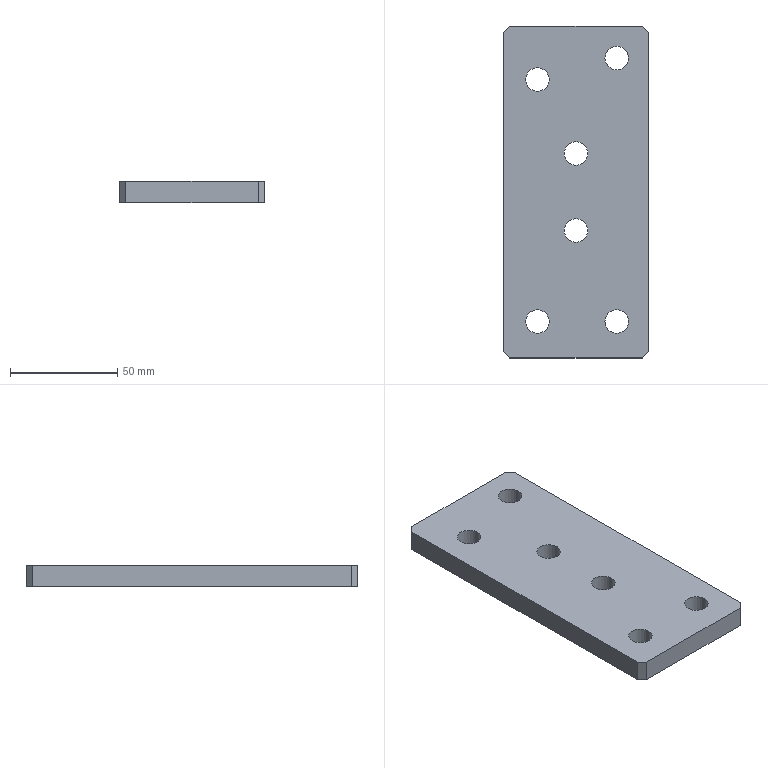Part | STEP file | 1_id186_x_t | 1 solid | 16 faces | box 68 x 155 x 10 mm | volume 99518 mm3 | plane 10 | cylinder 6 | commonest cylinder face diameters 11 x6
STEP:
#1=CARTESIAN_POINT('',(0.,0.,0.));
#2=DIRECTION('',(0.,0.,1.));
#3=DIRECTION('',(1.,0.,0.));
#4=AXIS2_PLACEMENT_3D('',#1,#2,#3);
#5=CARTESIAN_POINT('',(51.775,230.,100.11));
#6=VERTEX_POINT('',#5);
#7=CARTESIAN_POINT('',(46.275,230.,100.11));
#8=DIRECTION('',(0.,0.,-1.));
#9=DIRECTION('',(1.,0.,0.));
#10=AXIS2_PLACEMENT_3D('',#7,#8,#9);
#11=CIRCLE('',#10,5.5);
#12=CARTESIAN_POINT('',(46.275,230.,-100.11));
#13=DIRECTION('',(0.,0.,1.));
#14=DIRECTION('',(1.,0.,0.));
#15=AXIS2_PLACEMENT_3D('',#12,#13,#14);
#16=CYLINDRICAL_SURFACE('',#15,5.5);
#17=CARTESIAN_POINT('',(6.283,200.22));
#18=DIRECTION('',(-1.,0.));
#19=VECTOR('',#18,1.);
#20=LINE('',#17,#19);
#21=(GEOMETRIC_REPRESENTATION_CONTEXT(2)PARAMETRIC_REPRESENTATION_CONTEXT()REPRESENTATION_CONTEXT('',''));
#22=DEFINITIONAL_REPRESENTATION('',(#20),#21);
#23=PCURVE('',#16,#22);
#24=CARTESIAN_POINT('',(96.738,255.,100.11));
#25=DIRECTION('',(0.,0.,1.));
#26=DIRECTION('',(1.,0.,0.));
#27=AXIS2_PLACEMENT_3D('',#24,#25,#26);
#28=PLANE('',#27);
#29=CARTESIAN_POINT('',(-44.962,-25.));
#30=CARTESIAN_POINT('',(-44.962,-34.526));
#31=CARTESIAN_POINT('',(-53.212,-29.763));
#32=CARTESIAN_POINT('',(-61.462,-25.));
#33=CARTESIAN_POINT('',(-53.212,-20.237));
#34=CARTESIAN_POINT('',(-44.962,-15.474));
#35=CARTESIAN_POINT('',(-44.962,-25.));
#36=(BOUNDED_CURVE()B_SPLINE_CURVE(2,(#29,#30,#31,#32,#33,#34,#35),.UNSPECIFIED.,.T.,.F.)B_SPLINE_CURVE_WITH_KNOTS((1,2,2,2,2,1),(-2.094,0.,2.094,4.189,6.283,8.378),.UNSPECIFIED.)CURVE()GEOMETRIC_REPRESENTATION_ITEM()RATIONAL_B_SPLINE_CURVE((1.,0.5,1.,0.5,1.,0.5,1.))REPRESENTATION_ITEM(''));
#37=(GEOMETRIC_REPRESENTATION_CONTEXT(2)PARAMETRIC_REPRESENTATION_CONTEXT()REPRESENTATION_CONTEXT('',''));
#38=DEFINITIONAL_REPRESENTATION('',(#36),#37);
#39=PCURVE('',#28,#38);
#40=SURFACE_CURVE('',#11,(#23,#39),.PCURVE_S1.);
#41=EDGE_CURVE('',#6,#6,#40,.T.);
#42=ORIENTED_EDGE('',*,*,#41,.T.);
#43=CARTESIAN_POINT('',(51.775,230.,90.11));
#44=VERTEX_POINT('',#43);
#45=CARTESIAN_POINT('',(51.775,230.,90.11));
#46=CARTESIAN_POINT('',(51.775,230.,100.11));
#47=B_SPLINE_CURVE_WITH_KNOTS('',1,(#45,#46),.UNSPECIFIED.,.F.,.F.,(2,2),(190.22,200.22),.PIECEWISE_BEZIER_KNOTS.);
#48=CARTESIAN_POINT('',(0.,0.));
#49=DIRECTION('',(0.,1.));
#50=VECTOR('',#49,1.);
#51=LINE('',#48,#50);
#52=(GEOMETRIC_REPRESENTATION_CONTEXT(2)PARAMETRIC_REPRESENTATION_CONTEXT()REPRESENTATION_CONTEXT('',''));
#53=DEFINITIONAL_REPRESENTATION('',(#51),#52);
#54=PCURVE('',#16,#53);
#55=CARTESIAN_POINT('',(6.283,0.));
#56=DIRECTION('',(0.,1.));
#57=VECTOR('',#56,1.);
#58=LINE('',#55,#57);
#59=(GEOMETRIC_REPRESENTATION_CONTEXT(2)PARAMETRIC_REPRESENTATION_CONTEXT()REPRESENTATION_CONTEXT('',''));
#60=DEFINITIONAL_REPRESENTATION('',(#58),#59);
#61=PCURVE('',#16,#60);
#62=SEAM_CURVE('',#47,(#54,#61),.PCURVE_S1.);
#63=EDGE_CURVE('',#44,#6,#62,.T.);
#64=ORIENTED_EDGE('',*,*,#63,.F.);
#65=CARTESIAN_POINT('',(46.275,230.,90.11));
#66=DIRECTION('',(0.,0.,-1.));
#67=DIRECTION('',(1.,0.,0.));
#68=AXIS2_PLACEMENT_3D('',#65,#66,#67);
#69=CIRCLE('',#68,5.5);
#70=CARTESIAN_POINT('',(6.283,190.22));
#71=DIRECTION('',(-1.,0.));
#72=VECTOR('',#71,1.);
#73=LINE('',#70,#72);
#74=(GEOMETRIC_REPRESENTATION_CONTEXT(2)PARAMETRIC_REPRESENTATION_CONTEXT()REPRESENTATION_CONTEXT('',''));
#75=DEFINITIONAL_REPRESENTATION('',(#73),#74);
#76=PCURVE('',#16,#75);
#77=CARTESIAN_POINT('',(96.738,255.,90.11));
#78=DIRECTION('',(0.,0.,1.));
#79=DIRECTION('',(1.,0.,0.));
#80=AXIS2_PLACEMENT_3D('',#77,#78,#79);
#81=PLANE('',#80);
#82=CARTESIAN_POINT('',(-44.962,-25.));
#83=CARTESIAN_POINT('',(-44.962,-34.526));
#84=CARTESIAN_POINT('',(-53.212,-29.763));
#85=CARTESIAN_POINT('',(-61.462,-25.));
#86=CARTESIAN_POINT('',(-53.212,-20.237));
#87=CARTESIAN_POINT('',(-44.962,-15.474));
#88=CARTESIAN_POINT('',(-44.962,-25.));
#89=(BOUNDED_CURVE()B_SPLINE_CURVE(2,(#82,#83,#84,#85,#86,#87,#88),.UNSPECIFIED.,.T.,.F.)B_SPLINE_CURVE_WITH_KNOTS((1,2,2,2,2,1),(-2.094,0.,2.094,4.189,6.283,8.378),.UNSPECIFIED.)CURVE()GEOMETRIC_REPRESENTATION_ITEM()RATIONAL_B_SPLINE_CURVE((1.,0.5,1.,0.5,1.,0.5,1.))REPRESENTATION_ITEM(''));
#90=(GEOMETRIC_REPRESENTATION_CONTEXT(2)PARAMETRIC_REPRESENTATION_CONTEXT()REPRESENTATION_CONTEXT('',''));
#91=DEFINITIONAL_REPRESENTATION('',(#89),#90);
#92=PCURVE('',#81,#91);
#93=SURFACE_CURVE('',#69,(#76,#92),.PCURVE_S1.);
#94=EDGE_CURVE('',#44,#44,#93,.T.);
#95=ORIENTED_EDGE('',*,*,#94,.F.);
#96=ORIENTED_EDGE('',*,*,#63,.T.);
#97=EDGE_LOOP('',(#42,#64,#95,#96));
#98=FACE_BOUND('',#97,.F.);
#99=ADVANCED_FACE('',(#98),#16,.F.);
#100=CARTESIAN_POINT('',(30.275,252.,90.11));
#101=VERTEX_POINT('',#100);
#102=CARTESIAN_POINT('',(30.275,252.,100.11));
#103=VERTEX_POINT('',#102);
#104=CARTESIAN_POINT('',(30.275,252.,90.11));
#105=DIRECTION('',(0.,0.,1.));
#106=VECTOR('',#105,1.);
#107=LINE('',#104,#106);
#108=CARTESIAN_POINT('',(30.275,100.,100.11));
#109=DIRECTION('',(1.,0.,0.));
#110=DIRECTION('',(0.,-1.,0.));
#111=AXIS2_PLACEMENT_3D('',#108,#109,#110);
#112=PLANE('',#111);
#113=CARTESIAN_POINT('',(-152.,10.));
#114=DIRECTION('',(0.,-1.));
#115=VECTOR('',#114,1.);
#116=LINE('',#113,#115);
#117=(GEOMETRIC_REPRESENTATION_CONTEXT(2)PARAMETRIC_REPRESENTATION_CONTEXT()REPRESENTATION_CONTEXT('',''));
#118=DEFINITIONAL_REPRESENTATION('',(#116),#117);
#119=PCURVE('',#112,#118);
#120=CARTESIAN_POINT('',(65.006,286.731,100.11));
#121=DIRECTION('',(0.7071,-0.7071,0.));
#122=DIRECTION('',(-0.7071,-0.7071,0.));
#123=AXIS2_PLACEMENT_3D('',#120,#121,#122);
#124=PLANE('',#123);
#125=CARTESIAN_POINT('',(49.117,10.));
#126=DIRECTION('',(0.,-1.));
#127=VECTOR('',#126,1.);
#128=LINE('',#125,#127);
#129=(GEOMETRIC_REPRESENTATION_CONTEXT(2)PARAMETRIC_REPRESENTATION_CONTEXT()REPRESENTATION_CONTEXT('',''));
#130=DEFINITIONAL_REPRESENTATION('',(#128),#129);
#131=PCURVE('',#124,#130);
#132=SURFACE_CURVE('',#107,(#119,#131),.PCURVE_S1.);
#133=EDGE_CURVE('',#101,#103,#132,.T.);
#134=ORIENTED_EDGE('',*,*,#133,.F.);
#135=CARTESIAN_POINT('',(30.275,103.,90.11));
#136=VERTEX_POINT('',#135);
#137=CARTESIAN_POINT('',(30.275,252.,90.11));
#138=DIRECTION('',(0.,-1.,0.));
#139=VECTOR('',#138,1.);
#140=LINE('',#137,#139);
#141=CARTESIAN_POINT('',(-152.,10.));
#142=DIRECTION('',(1.,0.));
#143=VECTOR('',#142,1.);
#144=LINE('',#141,#143);
#145=(GEOMETRIC_REPRESENTATION_CONTEXT(2)PARAMETRIC_REPRESENTATION_CONTEXT()REPRESENTATION_CONTEXT('',''));
#146=DEFINITIONAL_REPRESENTATION('',(#144),#145);
#147=PCURVE('',#112,#146);
#148=CARTESIAN_POINT('',(-66.463,-3.));
#149=DIRECTION('',(0.,-1.));
#150=VECTOR('',#149,1.);
#151=LINE('',#148,#150);
#152=(GEOMETRIC_REPRESENTATION_CONTEXT(2)PARAMETRIC_REPRESENTATION_CONTEXT()REPRESENTATION_CONTEXT('',''));
#153=DEFINITIONAL_REPRESENTATION('',(#151),#152);
#154=PCURVE('',#81,#153);
#155=SURFACE_CURVE('',#140,(#147,#154),.PCURVE_S1.);
#156=EDGE_CURVE('',#101,#136,#155,.T.);
#157=ORIENTED_EDGE('',*,*,#156,.T.);
#158=CARTESIAN_POINT('',(30.275,103.,100.11));
#159=VERTEX_POINT('',#158);
#160=CARTESIAN_POINT('',(30.275,103.,90.11));
#161=DIRECTION('',(0.,0.,1.));
#162=VECTOR('',#161,1.);
#163=LINE('',#160,#162);
#164=CARTESIAN_POINT('',(-3.,10.));
#165=DIRECTION('',(0.,-1.));
#166=VECTOR('',#165,1.);
#167=LINE('',#164,#166);
#168=(GEOMETRIC_REPRESENTATION_CONTEXT(2)PARAMETRIC_REPRESENTATION_CONTEXT()REPRESENTATION_CONTEXT('',''));
#169=DEFINITIONAL_REPRESENTATION('',(#167),#168);
#170=PCURVE('',#112,#169);
#171=CARTESIAN_POINT('',(-12.494,145.769,100.11));
#172=DIRECTION('',(0.7071,0.7071,0.));
#173=DIRECTION('',(0.7071,-0.7071,0.));
#174=AXIS2_PLACEMENT_3D('',#171,#172,#173);
#175=PLANE('',#174);
#176=CARTESIAN_POINT('',(60.484,10.));
#177=DIRECTION('',(0.,-1.));
#178=VECTOR('',#177,1.);
#179=LINE('',#176,#178);
#180=(GEOMETRIC_REPRESENTATION_CONTEXT(2)PARAMETRIC_REPRESENTATION_CONTEXT()REPRESENTATION_CONTEXT('',''));
#181=DEFINITIONAL_REPRESENTATION('',(#179),#180);
#182=PCURVE('',#175,#181);
#183=SURFACE_CURVE('',#163,(#170,#182),.PCURVE_S1.);
#184=EDGE_CURVE('',#136,#159,#183,.T.);
#185=ORIENTED_EDGE('',*,*,#184,.T.);
#186=CARTESIAN_POINT('',(30.275,252.,100.11));
#187=DIRECTION('',(0.,-1.,0.));
#188=VECTOR('',#187,1.);
#189=LINE('',#186,#188);
#190=CARTESIAN_POINT('',(-152.,0.));
#191=DIRECTION('',(1.,0.));
#192=VECTOR('',#191,1.);
#193=LINE('',#190,#192);
#194=(GEOMETRIC_REPRESENTATION_CONTEXT(2)PARAMETRIC_REPRESENTATION_CONTEXT()REPRESENTATION_CONTEXT('',''));
#195=DEFINITIONAL_REPRESENTATION('',(#193),#194);
#196=PCURVE('',#112,#195);
#197=CARTESIAN_POINT('',(-66.463,-3.));
#198=DIRECTION('',(0.,-1.));
#199=VECTOR('',#198,1.);
#200=LINE('',#197,#199);
#201=(GEOMETRIC_REPRESENTATION_CONTEXT(2)PARAMETRIC_REPRESENTATION_CONTEXT()REPRESENTATION_CONTEXT('',''));
#202=DEFINITIONAL_REPRESENTATION('',(#200),#201);
#203=PCURVE('',#28,#202);
#204=SURFACE_CURVE('',#189,(#196,#203),.PCURVE_S1.);
#205=EDGE_CURVE('',#103,#159,#204,.T.);
#206=ORIENTED_EDGE('',*,*,#205,.F.);
#207=EDGE_LOOP('',(#134,#157,#185,#206));
#208=FACE_BOUND('',#207,.T.);
#209=ADVANCED_FACE('',(#208),#112,.F.);
#210=CARTESIAN_POINT('',(33.275,100.,90.11));
#211=VERTEX_POINT('',#210);
#212=CARTESIAN_POINT('',(33.275,100.,100.11));
#213=VERTEX_POINT('',#212);
#214=CARTESIAN_POINT('',(33.275,100.,90.11));
#215=DIRECTION('',(0.,0.,1.));
#216=VECTOR('',#215,1.);
#217=LINE('',#214,#216);
#218=CARTESIAN_POINT('',(64.727,10.));
#219=DIRECTION('',(0.,-1.));
#220=VECTOR('',#219,1.);
#221=LINE('',#218,#220);
#222=(GEOMETRIC_REPRESENTATION_CONTEXT(2)PARAMETRIC_REPRESENTATION_CONTEXT()REPRESENTATION_CONTEXT('',''));
#223=DEFINITIONAL_REPRESENTATION('',(#221),#222);
#224=PCURVE('',#175,#223);
#225=CARTESIAN_POINT('',(96.738,100.,100.11));
#226=DIRECTION('',(0.,1.,0.));
#227=DIRECTION('',(0.,0.,1.));
#228=AXIS2_PLACEMENT_3D('',#225,#226,#227);
#229=PLANE('',#228);
#230=CARTESIAN_POINT('',(-10.,-63.462));
#231=DIRECTION('',(1.,0.));
#232=VECTOR('',#231,1.);
#233=LINE('',#230,#232);
#234=(GEOMETRIC_REPRESENTATION_CONTEXT(2)PARAMETRIC_REPRESENTATION_CONTEXT()REPRESENTATION_CONTEXT('',''));
#235=DEFINITIONAL_REPRESENTATION('',(#233),#234);
#236=PCURVE('',#229,#235);
#237=SURFACE_CURVE('',#217,(#224,#236),.PCURVE_S1.);
#238=EDGE_CURVE('',#211,#213,#237,.T.);
#239=ORIENTED_EDGE('',*,*,#238,.T.);
#240=CARTESIAN_POINT('',(30.275,103.,100.11));
#241=DIRECTION('',(0.7071,-0.7071,0.));
#242=VECTOR('',#241,1.);
#243=LINE('',#240,#242);
#244=CARTESIAN_POINT('',(60.484,0.));
#245=DIRECTION('',(1.,0.));
#246=VECTOR('',#245,1.);
#247=LINE('',#244,#246);
#248=(GEOMETRIC_REPRESENTATION_CONTEXT(2)PARAMETRIC_REPRESENTATION_CONTEXT()REPRESENTATION_CONTEXT('',''));
#249=DEFINITIONAL_REPRESENTATION('',(#247),#248);
#250=PCURVE('',#175,#249);
#251=CARTESIAN_POINT('',(-66.463,-152.));
#252=DIRECTION('',(0.7071,-0.7071));
#253=VECTOR('',#252,1.);
#254=LINE('',#251,#253);
#255=(GEOMETRIC_REPRESENTATION_CONTEXT(2)PARAMETRIC_REPRESENTATION_CONTEXT()REPRESENTATION_CONTEXT('',''));
#256=DEFINITIONAL_REPRESENTATION('',(#254),#255);
#257=PCURVE('',#28,#256);
#258=SURFACE_CURVE('',#243,(#250,#257),.PCURVE_S1.);
#259=EDGE_CURVE('',#159,#213,#258,.T.);
#260=ORIENTED_EDGE('',*,*,#259,.F.);
#261=ORIENTED_EDGE('',*,*,#184,.F.);
#262=CARTESIAN_POINT('',(33.275,100.,90.11));
#263=DIRECTION('',(-0.7071,0.7071,0.));
#264=VECTOR('',#263,1.);
#265=LINE('',#262,#264);
#266=CARTESIAN_POINT('',(64.727,10.));
#267=DIRECTION('',(-1.,0.));
#268=VECTOR('',#267,1.);
#269=LINE('',#266,#268);
#270=(GEOMETRIC_REPRESENTATION_CONTEXT(2)PARAMETRIC_REPRESENTATION_CONTEXT()REPRESENTATION_CONTEXT('',''));
#271=DEFINITIONAL_REPRESENTATION('',(#269),#270);
#272=PCURVE('',#175,#271);
#273=CARTESIAN_POINT('',(-63.462,-155.));
#274=DIRECTION('',(-0.7071,0.7071));
#275=VECTOR('',#274,1.);
#276=LINE('',#273,#275);
#277=(GEOMETRIC_REPRESENTATION_CONTEXT(2)PARAMETRIC_REPRESENTATION_CONTEXT()REPRESENTATION_CONTEXT('',''));
#278=DEFINITIONAL_REPRESENTATION('',(#276),#277);
#279=PCURVE('',#81,#278);
#280=SURFACE_CURVE('',#265,(#272,#279),.PCURVE_S1.);
#281=EDGE_CURVE('',#211,#136,#280,.T.);
#282=ORIENTED_EDGE('',*,*,#281,.F.);
#283=EDGE_LOOP('',(#239,#260,#261,#282));
#284=FACE_BOUND('',#283,.T.);
#285=ADVANCED_FACE('',(#284),#175,.F.);
#286=CARTESIAN_POINT('',(95.275,100.,90.11));
#287=VERTEX_POINT('',#286);
#288=CARTESIAN_POINT('',(95.275,100.,100.11));
#289=VERTEX_POINT('',#288);
#290=CARTESIAN_POINT('',(95.275,100.,90.11));
#291=DIRECTION('',(0.,0.,1.));
#292=VECTOR('',#291,1.);
#293=LINE('',#290,#292);
#294=CARTESIAN_POINT('',(-10.,-1.462));
#295=DIRECTION('',(1.,0.));
#296=VECTOR('',#295,1.);
#297=LINE('',#294,#296);
#298=(GEOMETRIC_REPRESENTATION_CONTEXT(2)PARAMETRIC_REPRESENTATION_CONTEXT()REPRESENTATION_CONTEXT('',''));
#299=DEFINITIONAL_REPRESENTATION('',(#297),#298);
#300=PCURVE('',#229,#299);
#301=CARTESIAN_POINT('',(173.506,178.231,100.11));
#302=DIRECTION('',(-0.7071,0.7071,0.));
#303=DIRECTION('',(0.7071,0.7071,0.));
#304=AXIS2_PLACEMENT_3D('',#301,#302,#303);
#305=PLANE('',#304);
#306=CARTESIAN_POINT('',(-110.636,10.));
#307=DIRECTION('',(0.,-1.));
#308=VECTOR('',#307,1.);
#309=LINE('',#306,#308);
#310=(GEOMETRIC_REPRESENTATION_CONTEXT(2)PARAMETRIC_REPRESENTATION_CONTEXT()REPRESENTATION_CONTEXT('',''));
#311=DEFINITIONAL_REPRESENTATION('',(#309),#310);
#312=PCURVE('',#305,#311);
#313=SURFACE_CURVE('',#293,(#300,#312),.PCURVE_S1.);
#314=EDGE_CURVE('',#287,#289,#313,.T.);
#315=ORIENTED_EDGE('',*,*,#314,.T.);
#316=CARTESIAN_POINT('',(33.275,100.,100.11));
#317=DIRECTION('',(1.,0.,0.));
#318=VECTOR('',#317,1.);
#319=LINE('',#316,#318);
#320=CARTESIAN_POINT('',(0.,-63.462));
#321=DIRECTION('',(0.,1.));
#322=VECTOR('',#321,1.);
#323=LINE('',#320,#322);
#324=(GEOMETRIC_REPRESENTATION_CONTEXT(2)PARAMETRIC_REPRESENTATION_CONTEXT()REPRESENTATION_CONTEXT('',''));
#325=DEFINITIONAL_REPRESENTATION('',(#323),#324);
#326=PCURVE('',#229,#325);
#327=CARTESIAN_POINT('',(-63.462,-155.));
#328=DIRECTION('',(1.,0.));
#329=VECTOR('',#328,1.);
#330=LINE('',#327,#329);
#331=(GEOMETRIC_REPRESENTATION_CONTEXT(2)PARAMETRIC_REPRESENTATION_CONTEXT()REPRESENTATION_CONTEXT('',''));
#332=DEFINITIONAL_REPRESENTATION('',(#330),#331);
#333=PCURVE('',#28,#332);
#334=SURFACE_CURVE('',#319,(#326,#333),.PCURVE_S1.);
#335=EDGE_CURVE('',#213,#289,#334,.T.);
#336=ORIENTED_EDGE('',*,*,#335,.F.);
#337=ORIENTED_EDGE('',*,*,#238,.F.);
#338=CARTESIAN_POINT('',(33.275,100.,90.11));
#339=DIRECTION('',(1.,0.,0.));
#340=VECTOR('',#339,1.);
#341=LINE('',#338,#340);
#342=CARTESIAN_POINT('',(-10.,-63.462));
#343=DIRECTION('',(0.,1.));
#344=VECTOR('',#343,1.);
#345=LINE('',#342,#344);
#346=(GEOMETRIC_REPRESENTATION_CONTEXT(2)PARAMETRIC_REPRESENTATION_CONTEXT()REPRESENTATION_CONTEXT('',''));
#347=DEFINITIONAL_REPRESENTATION('',(#345),#346);
#348=PCURVE('',#229,#347);
#349=CARTESIAN_POINT('',(-63.462,-155.));
#350=DIRECTION('',(1.,0.));
#351=VECTOR('',#350,1.);
#352=LINE('',#349,#351);
#353=(GEOMETRIC_REPRESENTATION_CONTEXT(2)PARAMETRIC_REPRESENTATION_CONTEXT()REPRESENTATION_CONTEXT('',''));
#354=DEFINITIONAL_REPRESENTATION('',(#352),#353);
#355=PCURVE('',#81,#354);
#356=SURFACE_CURVE('',#341,(#348,#355),.PCURVE_S1.);
#357=EDGE_CURVE('',#211,#287,#356,.T.);
#358=ORIENTED_EDGE('',*,*,#357,.T.);
#359=EDGE_LOOP('',(#315,#336,#337,#358));
#360=FACE_BOUND('',#359,.T.);
#361=ADVANCED_FACE('',(#360),#229,.F.);
#362=CARTESIAN_POINT('',(98.275,103.,90.11));
#363=VERTEX_POINT('',#362);
#364=CARTESIAN_POINT('',(98.275,103.,100.11));
#365=VERTEX_POINT('',#364);
#366=CARTESIAN_POINT('',(98.275,103.,90.11));
#367=DIRECTION('',(0.,0.,1.));
#368=VECTOR('',#367,1.);
#369=LINE('',#366,#368);
#370=CARTESIAN_POINT('',(-106.393,10.));
#371=DIRECTION('',(0.,-1.));
#372=VECTOR('',#371,1.);
#373=LINE('',#370,#372);
#374=(GEOMETRIC_REPRESENTATION_CONTEXT(2)PARAMETRIC_REPRESENTATION_CONTEXT()REPRESENTATION_CONTEXT('',''));
#375=DEFINITIONAL_REPRESENTATION('',(#373),#374);
#376=PCURVE('',#305,#375);
#377=CARTESIAN_POINT('',(98.275,100.,100.11));
#378=DIRECTION('',(-1.,0.,0.));
#379=DIRECTION('',(0.,1.,0.));
#380=AXIS2_PLACEMENT_3D('',#377,#378,#379);
#381=PLANE('',#380);
#382=CARTESIAN_POINT('',(3.,10.));
#383=DIRECTION('',(0.,-1.));
#384=VECTOR('',#383,1.);
#385=LINE('',#382,#384);
#386=(GEOMETRIC_REPRESENTATION_CONTEXT(2)PARAMETRIC_REPRESENTATION_CONTEXT()REPRESENTATION_CONTEXT('',''));
#387=DEFINITIONAL_REPRESENTATION('',(#385),#386);
#388=PCURVE('',#381,#387);
#389=SURFACE_CURVE('',#369,(#376,#388),.PCURVE_S1.);
#390=EDGE_CURVE('',#363,#365,#389,.T.);
#391=ORIENTED_EDGE('',*,*,#390,.T.);
#392=CARTESIAN_POINT('',(95.275,100.,100.11));
#393=DIRECTION('',(0.7071,0.7071,0.));
#394=VECTOR('',#393,1.);
#395=LINE('',#392,#394);
#396=CARTESIAN_POINT('',(-110.636,0.));
#397=DIRECTION('',(1.,0.));
#398=VECTOR('',#397,1.);
#399=LINE('',#396,#398);
#400=(GEOMETRIC_REPRESENTATION_CONTEXT(2)PARAMETRIC_REPRESENTATION_CONTEXT()REPRESENTATION_CONTEXT('',''));
#401=DEFINITIONAL_REPRESENTATION('',(#399),#400);
#402=PCURVE('',#305,#401);
#403=CARTESIAN_POINT('',(-1.462,-155.));
#404=DIRECTION('',(0.7071,0.7071));
#405=VECTOR('',#404,1.);
#406=LINE('',#403,#405);
#407=(GEOMETRIC_REPRESENTATION_CONTEXT(2)PARAMETRIC_REPRESENTATION_CONTEXT()REPRESENTATION_CONTEXT('',''));
#408=DEFINITIONAL_REPRESENTATION('',(#406),#407);
#409=PCURVE('',#28,#408);
#410=SURFACE_CURVE('',#395,(#402,#409),.PCURVE_S1.);
#411=EDGE_CURVE('',#289,#365,#410,.T.);
#412=ORIENTED_EDGE('',*,*,#411,.F.);
#413=ORIENTED_EDGE('',*,*,#314,.F.);
#414=CARTESIAN_POINT('',(98.275,103.,90.11));
#415=DIRECTION('',(-0.7071,-0.7071,0.));
#416=VECTOR('',#415,1.);
#417=LINE('',#414,#416);
#418=CARTESIAN_POINT('',(-106.393,10.));
#419=DIRECTION('',(-1.,0.));
#420=VECTOR('',#419,1.);
#421=LINE('',#418,#420);
#422=(GEOMETRIC_REPRESENTATION_CONTEXT(2)PARAMETRIC_REPRESENTATION_CONTEXT()REPRESENTATION_CONTEXT('',''));
#423=DEFINITIONAL_REPRESENTATION('',(#421),#422);
#424=PCURVE('',#305,#423);
#425=CARTESIAN_POINT('',(1.538,-152.));
#426=DIRECTION('',(-0.7071,-0.7071));
#427=VECTOR('',#426,1.);
#428=LINE('',#425,#427);
#429=(GEOMETRIC_REPRESENTATION_CONTEXT(2)PARAMETRIC_REPRESENTATION_CONTEXT()REPRESENTATION_CONTEXT('',''));
#430=DEFINITIONAL_REPRESENTATION('',(#428),#429);
#431=PCURVE('',#81,#430);
#432=SURFACE_CURVE('',#417,(#424,#431),.PCURVE_S1.);
#433=EDGE_CURVE('',#363,#287,#432,.T.);
#434=ORIENTED_EDGE('',*,*,#433,.F.);
#435=EDGE_LOOP('',(#391,#412,#413,#434));
#436=FACE_BOUND('',#435,.T.);
#437=ADVANCED_FACE('',(#436),#305,.F.);
#438=CARTESIAN_POINT('',(98.275,252.,90.11));
#439=VERTEX_POINT('',#438);
#440=CARTESIAN_POINT('',(98.275,252.,100.11));
#441=VERTEX_POINT('',#440);
#442=CARTESIAN_POINT('',(98.275,252.,90.11));
#443=DIRECTION('',(0.,0.,1.));
#444=VECTOR('',#443,1.);
#445=LINE('',#442,#444);
#446=CARTESIAN_POINT('',(152.,10.));
#447=DIRECTION('',(0.,-1.));
#448=VECTOR('',#447,1.);
#449=LINE('',#446,#448);
#450=(GEOMETRIC_REPRESENTATION_CONTEXT(2)PARAMETRIC_REPRESENTATION_CONTEXT()REPRESENTATION_CONTEXT('',''));
#451=DEFINITIONAL_REPRESENTATION('',(#449),#450);
#452=PCURVE('',#381,#451);
#453=CARTESIAN_POINT('',(96.006,254.269,100.11));
#454=DIRECTION('',(-0.7071,-0.7071,0.));
#455=DIRECTION('',(-0.7071,0.7071,0.));
#456=AXIS2_PLACEMENT_3D('',#453,#454,#455);
#457=PLANE('',#456);
#458=CARTESIAN_POINT('',(-3.208,10.));
#459=DIRECTION('',(0.,-1.));
#460=VECTOR('',#459,1.);
#461=LINE('',#458,#460);
#462=(GEOMETRIC_REPRESENTATION_CONTEXT(2)PARAMETRIC_REPRESENTATION_CONTEXT()REPRESENTATION_CONTEXT('',''));
#463=DEFINITIONAL_REPRESENTATION('',(#461),#462);
#464=PCURVE('',#457,#463);
#465=SURFACE_CURVE('',#445,(#452,#464),.PCURVE_S1.);
#466=EDGE_CURVE('',#439,#441,#465,.T.);
#467=ORIENTED_EDGE('',*,*,#466,.T.);
#468=CARTESIAN_POINT('',(98.275,103.,100.11));
#469=DIRECTION('',(0.,1.,0.));
#470=VECTOR('',#469,1.);
#471=LINE('',#468,#470);
#472=CARTESIAN_POINT('',(3.,0.));
#473=DIRECTION('',(1.,0.));
#474=VECTOR('',#473,1.);
#475=LINE('',#472,#474);
#476=(GEOMETRIC_REPRESENTATION_CONTEXT(2)PARAMETRIC_REPRESENTATION_CONTEXT()REPRESENTATION_CONTEXT('',''));
#477=DEFINITIONAL_REPRESENTATION('',(#475),#476);
#478=PCURVE('',#381,#477);
#479=CARTESIAN_POINT('',(1.538,-152.));
#480=DIRECTION('',(0.,1.));
#481=VECTOR('',#480,1.);
#482=LINE('',#479,#481);
#483=(GEOMETRIC_REPRESENTATION_CONTEXT(2)PARAMETRIC_REPRESENTATION_CONTEXT()REPRESENTATION_CONTEXT('',''));
#484=DEFINITIONAL_REPRESENTATION('',(#482),#483);
#485=PCURVE('',#28,#484);
#486=SURFACE_CURVE('',#471,(#478,#485),.PCURVE_S1.);
#487=EDGE_CURVE('',#365,#441,#486,.T.);
#488=ORIENTED_EDGE('',*,*,#487,.F.);
#489=ORIENTED_EDGE('',*,*,#390,.F.);
#490=CARTESIAN_POINT('',(98.275,103.,90.11));
#491=DIRECTION('',(0.,1.,0.));
#492=VECTOR('',#491,1.);
#493=LINE('',#490,#492);
#494=CARTESIAN_POINT('',(3.,10.));
#495=DIRECTION('',(1.,0.));
#496=VECTOR('',#495,1.);
#497=LINE('',#494,#496);
#498=(GEOMETRIC_REPRESENTATION_CONTEXT(2)PARAMETRIC_REPRESENTATION_CONTEXT()REPRESENTATION_CONTEXT('',''));
#499=DEFINITIONAL_REPRESENTATION('',(#497),#498);
#500=PCURVE('',#381,#499);
#501=CARTESIAN_POINT('',(1.538,-152.));
#502=DIRECTION('',(0.,1.));
#503=VECTOR('',#502,1.);
#504=LINE('',#501,#503);
#505=(GEOMETRIC_REPRESENTATION_CONTEXT(2)PARAMETRIC_REPRESENTATION_CONTEXT()REPRESENTATION_CONTEXT('',''));
#506=DEFINITIONAL_REPRESENTATION('',(#504),#505);
#507=PCURVE('',#81,#506);
#508=SURFACE_CURVE('',#493,(#500,#507),.PCURVE_S1.);
#509=EDGE_CURVE('',#363,#439,#508,.T.);
#510=ORIENTED_EDGE('',*,*,#509,.T.);
#511=EDGE_LOOP('',(#467,#488,#489,#510));
#512=FACE_BOUND('',#511,.T.);
#513=ADVANCED_FACE('',(#512),#381,.F.);
#514=CARTESIAN_POINT('',(95.275,255.,90.11));
#515=VERTEX_POINT('',#514);
#516=CARTESIAN_POINT('',(95.275,255.,100.11));
#517=VERTEX_POINT('',#516);
#518=CARTESIAN_POINT('',(95.275,255.,90.11));
#519=DIRECTION('',(0.,0.,1.));
#520=VECTOR('',#519,1.);
#521=LINE('',#518,#520);
#522=CARTESIAN_POINT('',(1.034,10.));
#523=DIRECTION('',(0.,-1.));
#524=VECTOR('',#523,1.);
#525=LINE('',#522,#524);
#526=(GEOMETRIC_REPRESENTATION_CONTEXT(2)PARAMETRIC_REPRESENTATION_CONTEXT()REPRESENTATION_CONTEXT('',''));
#527=DEFINITIONAL_REPRESENTATION('',(#525),#526);
#528=PCURVE('',#457,#527);
#529=CARTESIAN_POINT('',(31.813,255.,100.11));
#530=DIRECTION('',(0.,-1.,0.));
#531=DIRECTION('',(0.,0.,-1.));
#532=AXIS2_PLACEMENT_3D('',#529,#530,#531);
#533=PLANE('',#532);
#534=CARTESIAN_POINT('',(10.,63.462));
#535=DIRECTION('',(-1.,0.));
#536=VECTOR('',#535,1.);
#537=LINE('',#534,#536);
#538=(GEOMETRIC_REPRESENTATION_CONTEXT(2)PARAMETRIC_REPRESENTATION_CONTEXT()REPRESENTATION_CONTEXT('',''));
#539=DEFINITIONAL_REPRESENTATION('',(#537),#538);
#540=PCURVE('',#533,#539);
#541=SURFACE_CURVE('',#521,(#528,#540),.PCURVE_S1.);
#542=EDGE_CURVE('',#515,#517,#541,.T.);
#543=ORIENTED_EDGE('',*,*,#542,.T.);
#544=CARTESIAN_POINT('',(98.275,252.,100.11));
#545=DIRECTION('',(-0.7071,0.7071,0.));
#546=VECTOR('',#545,1.);
#547=LINE('',#544,#546);
#548=CARTESIAN_POINT('',(-3.208,0.));
#549=DIRECTION('',(1.,0.));
#550=VECTOR('',#549,1.);
#551=LINE('',#548,#550);
#552=(GEOMETRIC_REPRESENTATION_CONTEXT(2)PARAMETRIC_REPRESENTATION_CONTEXT()REPRESENTATION_CONTEXT('',''));
#553=DEFINITIONAL_REPRESENTATION('',(#551),#552);
#554=PCURVE('',#457,#553);
#555=CARTESIAN_POINT('',(1.538,-3.));
#556=DIRECTION('',(-0.7071,0.7071));
#557=VECTOR('',#556,1.);
#558=LINE('',#555,#557);
#559=(GEOMETRIC_REPRESENTATION_CONTEXT(2)PARAMETRIC_REPRESENTATION_CONTEXT()REPRESENTATION_CONTEXT('',''));
#560=DEFINITIONAL_REPRESENTATION('',(#558),#559);
#561=PCURVE('',#28,#560);
#562=SURFACE_CURVE('',#547,(#554,#561),.PCURVE_S1.);
#563=EDGE_CURVE('',#441,#517,#562,.T.);
#564=ORIENTED_EDGE('',*,*,#563,.F.);
#565=ORIENTED_EDGE('',*,*,#466,.F.);
#566=CARTESIAN_POINT('',(95.275,255.,90.11));
#567=DIRECTION('',(0.7071,-0.7071,0.));
#568=VECTOR('',#567,1.);
#569=LINE('',#566,#568);
#570=CARTESIAN_POINT('',(1.034,10.));
#571=DIRECTION('',(-1.,0.));
#572=VECTOR('',#571,1.);
#573=LINE('',#570,#572);
#574=(GEOMETRIC_REPRESENTATION_CONTEXT(2)PARAMETRIC_REPRESENTATION_CONTEXT()REPRESENTATION_CONTEXT('',''));
#575=DEFINITIONAL_REPRESENTATION('',(#573),#574);
#576=PCURVE('',#457,#575);
#577=CARTESIAN_POINT('',(-1.462,0.));
#578=DIRECTION('',(0.7071,-0.7071));
#579=VECTOR('',#578,1.);
#580=LINE('',#577,#579);
#581=(GEOMETRIC_REPRESENTATION_CONTEXT(2)PARAMETRIC_REPRESENTATION_CONTEXT()REPRESENTATION_CONTEXT('',''));
#582=DEFINITIONAL_REPRESENTATION('',(#580),#581);
#583=PCURVE('',#81,#582);
#584=SURFACE_CURVE('',#569,(#576,#583),.PCURVE_S1.);
#585=EDGE_CURVE('',#515,#439,#584,.T.);
#586=ORIENTED_EDGE('',*,*,#585,.F.);
#587=EDGE_LOOP('',(#543,#564,#565,#586));
#588=FACE_BOUND('',#587,.T.);
#589=ADVANCED_FACE('',(#588),#457,.F.);
#590=CARTESIAN_POINT('',(33.275,255.,90.11));
#591=VERTEX_POINT('',#590);
#592=CARTESIAN_POINT('',(33.275,255.,100.11));
#593=VERTEX_POINT('',#592);
#594=CARTESIAN_POINT('',(33.275,255.,90.11));
#595=DIRECTION('',(0.,0.,1.));
#596=VECTOR('',#595,1.);
#597=LINE('',#594,#596);
#598=CARTESIAN_POINT('',(10.,1.462));
#599=DIRECTION('',(-1.,0.));
#600=VECTOR('',#599,1.);
#601=LINE('',#598,#600);
#602=(GEOMETRIC_REPRESENTATION_CONTEXT(2)PARAMETRIC_REPRESENTATION_CONTEXT()REPRESENTATION_CONTEXT('',''));
#603=DEFINITIONAL_REPRESENTATION('',(#601),#602);
#604=PCURVE('',#533,#603);
#605=CARTESIAN_POINT('',(44.875,10.));
#606=DIRECTION('',(0.,-1.));
#607=VECTOR('',#606,1.);
#608=LINE('',#605,#607);
#609=(GEOMETRIC_REPRESENTATION_CONTEXT(2)PARAMETRIC_REPRESENTATION_CONTEXT()REPRESENTATION_CONTEXT('',''));
#610=DEFINITIONAL_REPRESENTATION('',(#608),#609);
#611=PCURVE('',#124,#610);
#612=SURFACE_CURVE('',#597,(#604,#611),.PCURVE_S1.);
#613=EDGE_CURVE('',#591,#593,#612,.T.);
#614=ORIENTED_EDGE('',*,*,#613,.T.);
#615=CARTESIAN_POINT('',(95.275,255.,100.11));
#616=DIRECTION('',(-1.,0.,0.));
#617=VECTOR('',#616,1.);
#618=LINE('',#615,#617);
#619=CARTESIAN_POINT('',(0.,63.462));
#620=DIRECTION('',(0.,-1.));
#621=VECTOR('',#620,1.);
#622=LINE('',#619,#621);
#623=(GEOMETRIC_REPRESENTATION_CONTEXT(2)PARAMETRIC_REPRESENTATION_CONTEXT()REPRESENTATION_CONTEXT('',''));
#624=DEFINITIONAL_REPRESENTATION('',(#622),#623);
#625=PCURVE('',#533,#624);
#626=CARTESIAN_POINT('',(-1.462,0.));
#627=DIRECTION('',(-1.,0.));
#628=VECTOR('',#627,1.);
#629=LINE('',#626,#628);
#630=(GEOMETRIC_REPRESENTATION_CONTEXT(2)PARAMETRIC_REPRESENTATION_CONTEXT()REPRESENTATION_CONTEXT('',''));
#631=DEFINITIONAL_REPRESENTATION('',(#629),#630);
#632=PCURVE('',#28,#631);
#633=SURFACE_CURVE('',#618,(#625,#632),.PCURVE_S1.);
#634=EDGE_CURVE('',#517,#593,#633,.T.);
#635=ORIENTED_EDGE('',*,*,#634,.F.);
#636=ORIENTED_EDGE('',*,*,#542,.F.);
#637=CARTESIAN_POINT('',(95.275,255.,90.11));
#638=DIRECTION('',(-1.,0.,0.));
#639=VECTOR('',#638,1.);
#640=LINE('',#637,#639);
#641=CARTESIAN_POINT('',(10.,63.462));
#642=DIRECTION('',(0.,-1.));
#643=VECTOR('',#642,1.);
#644=LINE('',#641,#643);
#645=(GEOMETRIC_REPRESENTATION_CONTEXT(2)PARAMETRIC_REPRESENTATION_CONTEXT()REPRESENTATION_CONTEXT('',''));
#646=DEFINITIONAL_REPRESENTATION('',(#644),#645);
#647=PCURVE('',#533,#646);
#648=CARTESIAN_POINT('',(-1.462,0.));
#649=DIRECTION('',(-1.,0.));
#650=VECTOR('',#649,1.);
#651=LINE('',#648,#650);
#652=(GEOMETRIC_REPRESENTATION_CONTEXT(2)PARAMETRIC_REPRESENTATION_CONTEXT()REPRESENTATION_CONTEXT('',''));
#653=DEFINITIONAL_REPRESENTATION('',(#651),#652);
#654=PCURVE('',#81,#653);
#655=SURFACE_CURVE('',#640,(#647,#654),.PCURVE_S1.);
#656=EDGE_CURVE('',#515,#591,#655,.T.);
#657=ORIENTED_EDGE('',*,*,#656,.T.);
#658=EDGE_LOOP('',(#614,#635,#636,#657));
#659=FACE_BOUND('',#658,.T.);
#660=ADVANCED_FACE('',(#659),#533,.F.);
#661=ORIENTED_EDGE('',*,*,#133,.T.);
#662=CARTESIAN_POINT('',(33.275,255.,100.11));
#663=DIRECTION('',(-0.7071,-0.7071,0.));
#664=VECTOR('',#663,1.);
#665=LINE('',#662,#664);
#666=CARTESIAN_POINT('',(44.875,0.));
#667=DIRECTION('',(1.,0.));
#668=VECTOR('',#667,1.);
#669=LINE('',#666,#668);
#670=(GEOMETRIC_REPRESENTATION_CONTEXT(2)PARAMETRIC_REPRESENTATION_CONTEXT()REPRESENTATION_CONTEXT('',''));
#671=DEFINITIONAL_REPRESENTATION('',(#669),#670);
#672=PCURVE('',#124,#671);
#673=CARTESIAN_POINT('',(-63.462,0.));
#674=DIRECTION('',(-0.7071,-0.7071));
#675=VECTOR('',#674,1.);
#676=LINE('',#673,#675);
#677=(GEOMETRIC_REPRESENTATION_CONTEXT(2)PARAMETRIC_REPRESENTATION_CONTEXT()REPRESENTATION_CONTEXT('',''));
#678=DEFINITIONAL_REPRESENTATION('',(#676),#677);
#679=PCURVE('',#28,#678);
#680=SURFACE_CURVE('',#665,(#672,#679),.PCURVE_S1.);
#681=EDGE_CURVE('',#593,#103,#680,.T.);
#682=ORIENTED_EDGE('',*,*,#681,.F.);
#683=ORIENTED_EDGE('',*,*,#613,.F.);
#684=CARTESIAN_POINT('',(30.275,252.,90.11));
#685=DIRECTION('',(0.7071,0.7071,0.));
#686=VECTOR('',#685,1.);
#687=LINE('',#684,#686);
#688=CARTESIAN_POINT('',(49.117,10.));
#689=DIRECTION('',(-1.,0.));
#690=VECTOR('',#689,1.);
#691=LINE('',#688,#690);
#692=(GEOMETRIC_REPRESENTATION_CONTEXT(2)PARAMETRIC_REPRESENTATION_CONTEXT()REPRESENTATION_CONTEXT('',''));
#693=DEFINITIONAL_REPRESENTATION('',(#691),#692);
#694=PCURVE('',#124,#693);
#695=CARTESIAN_POINT('',(-66.463,-3.));
#696=DIRECTION('',(0.7071,0.7071));
#697=VECTOR('',#696,1.);
#698=LINE('',#695,#697);
#699=(GEOMETRIC_REPRESENTATION_CONTEXT(2)PARAMETRIC_REPRESENTATION_CONTEXT()REPRESENTATION_CONTEXT('',''));
#700=DEFINITIONAL_REPRESENTATION('',(#698),#699);
#701=PCURVE('',#81,#700);
#702=SURFACE_CURVE('',#687,(#694,#701),.PCURVE_S1.);
#703=EDGE_CURVE('',#101,#591,#702,.T.);
#704=ORIENTED_EDGE('',*,*,#703,.F.);
#705=EDGE_LOOP('',(#661,#682,#683,#704));
#706=FACE_BOUND('',#705,.T.);
#707=ADVANCED_FACE('',(#706),#124,.F.);
#708=CARTESIAN_POINT('',(58.775,159.5,90.11));
#709=VERTEX_POINT('',#708);
#710=CARTESIAN_POINT('',(64.275,159.5,90.11));
#711=DIRECTION('',(0.,0.,1.));
#712=DIRECTION('',(-1.,0.,0.));
#713=AXIS2_PLACEMENT_3D('',#710,#711,#712);
#714=CIRCLE('',#713,5.5);
#715=CARTESIAN_POINT('',(64.275,159.5,100.11));
#716=DIRECTION('',(0.,0.,-1.));
#717=DIRECTION('',(-1.,0.,0.));
#718=AXIS2_PLACEMENT_3D('',#715,#716,#717);
#719=CYLINDRICAL_SURFACE('',#718,5.5);
#720=CARTESIAN_POINT('',(6.283,10.));
#721=DIRECTION('',(-1.,0.));
#722=VECTOR('',#721,1.);
#723=LINE('',#720,#722);
#724=(GEOMETRIC_REPRESENTATION_CONTEXT(2)PARAMETRIC_REPRESENTATION_CONTEXT()REPRESENTATION_CONTEXT('',''));
#725=DEFINITIONAL_REPRESENTATION('',(#723),#724);
#726=PCURVE('',#719,#725);
#727=CARTESIAN_POINT('',(-32.463,-95.5));
#728=DIRECTION('',(-1.,0.));
#729=AXIS2_PLACEMENT_2D('',#727,#728);
#730=CIRCLE('',#729,5.5);
#731=(GEOMETRIC_REPRESENTATION_CONTEXT(2)PARAMETRIC_REPRESENTATION_CONTEXT()REPRESENTATION_CONTEXT('',''));
#732=DEFINITIONAL_REPRESENTATION('',(#730),#731);
#733=PCURVE('',#81,#732);
#734=SURFACE_CURVE('',#714,(#726,#733),.PCURVE_S1.);
#735=EDGE_CURVE('',#709,#709,#734,.T.);
#736=ORIENTED_EDGE('',*,*,#735,.T.);
#737=CARTESIAN_POINT('',(58.775,159.5,100.11));
#738=VERTEX_POINT('',#737);
#739=CARTESIAN_POINT('',(58.775,159.5,100.11));
#740=CARTESIAN_POINT('',(58.775,159.5,90.11));
#741=B_SPLINE_CURVE_WITH_KNOTS('',1,(#739,#740),.UNSPECIFIED.,.F.,.F.,(2,2),(0.,10.),.PIECEWISE_BEZIER_KNOTS.);
#742=CARTESIAN_POINT('',(0.,0.));
#743=DIRECTION('',(0.,1.));
#744=VECTOR('',#743,1.);
#745=LINE('',#742,#744);
#746=(GEOMETRIC_REPRESENTATION_CONTEXT(2)PARAMETRIC_REPRESENTATION_CONTEXT()REPRESENTATION_CONTEXT('',''));
#747=DEFINITIONAL_REPRESENTATION('',(#745),#746);
#748=PCURVE('',#719,#747);
#749=CARTESIAN_POINT('',(6.283,0.));
#750=DIRECTION('',(0.,1.));
#751=VECTOR('',#750,1.);
#752=LINE('',#749,#751);
#753=(GEOMETRIC_REPRESENTATION_CONTEXT(2)PARAMETRIC_REPRESENTATION_CONTEXT()REPRESENTATION_CONTEXT('',''));
#754=DEFINITIONAL_REPRESENTATION('',(#752),#753);
#755=PCURVE('',#719,#754);
#756=SEAM_CURVE('',#741,(#748,#755),.PCURVE_S1.);
#757=EDGE_CURVE('',#738,#709,#756,.T.);
#758=ORIENTED_EDGE('',*,*,#757,.F.);
#759=CARTESIAN_POINT('',(69.775,159.5,100.11));
#760=VERTEX_POINT('',#759);
#761=CARTESIAN_POINT('',(64.275,159.5,100.11));
#762=DIRECTION('',(0.,0.,-1.));
#763=DIRECTION('',(1.,0.,0.));
#764=AXIS2_PLACEMENT_3D('',#761,#762,#763);
#765=CIRCLE('',#764,5.5);
#766=CARTESIAN_POINT('',(-3.142,0.));
#767=DIRECTION('',(1.,0.));
#768=VECTOR('',#767,1.);
#769=LINE('',#766,#768);
#770=(GEOMETRIC_REPRESENTATION_CONTEXT(2)PARAMETRIC_REPRESENTATION_CONTEXT()REPRESENTATION_CONTEXT('',''));
#771=DEFINITIONAL_REPRESENTATION('',(#769),#770);
#772=PCURVE('',#719,#771);
#773=CARTESIAN_POINT('',(-26.963,-95.5));
#774=CARTESIAN_POINT('',(-26.963,-105.026));
#775=CARTESIAN_POINT('',(-35.213,-100.263));
#776=CARTESIAN_POINT('',(-43.463,-95.5));
#777=CARTESIAN_POINT('',(-35.213,-90.737));
#778=CARTESIAN_POINT('',(-26.963,-85.974));
#779=CARTESIAN_POINT('',(-26.963,-95.5));
#780=(BOUNDED_CURVE()B_SPLINE_CURVE(2,(#773,#774,#775,#776,#777,#778,#779),.UNSPECIFIED.,.T.,.F.)B_SPLINE_CURVE_WITH_KNOTS((1,2,2,2,2,1),(-2.094,0.,2.094,4.189,6.283,8.378),.UNSPECIFIED.)CURVE()GEOMETRIC_REPRESENTATION_ITEM()RATIONAL_B_SPLINE_CURVE((1.,0.5,1.,0.5,1.,0.5,1.))REPRESENTATION_ITEM(''));
#781=(GEOMETRIC_REPRESENTATION_CONTEXT(2)PARAMETRIC_REPRESENTATION_CONTEXT()REPRESENTATION_CONTEXT('',''));
#782=DEFINITIONAL_REPRESENTATION('',(#780),#781);
#783=PCURVE('',#28,#782);
#784=SURFACE_CURVE('',#765,(#772,#783),.PCURVE_S1.);
#785=EDGE_CURVE('',#738,#760,#784,.T.);
#786=ORIENTED_EDGE('',*,*,#785,.T.);
#787=CARTESIAN_POINT('',(64.275,159.5,100.11));
#788=DIRECTION('',(0.,0.,-1.));
#789=DIRECTION('',(1.,0.,0.));
#790=AXIS2_PLACEMENT_3D('',#787,#788,#789);
#791=CIRCLE('',#790,5.5);
#792=CARTESIAN_POINT('',(3.142,0.));
#793=DIRECTION('',(1.,0.));
#794=VECTOR('',#793,1.);
#795=LINE('',#792,#794);
#796=(GEOMETRIC_REPRESENTATION_CONTEXT(2)PARAMETRIC_REPRESENTATION_CONTEXT()REPRESENTATION_CONTEXT('',''));
#797=DEFINITIONAL_REPRESENTATION('',(#795),#796);
#798=PCURVE('',#719,#797);
#799=CARTESIAN_POINT('',(-26.963,-95.5));
#800=CARTESIAN_POINT('',(-26.963,-105.026));
#801=CARTESIAN_POINT('',(-35.213,-100.263));
#802=CARTESIAN_POINT('',(-43.463,-95.5));
#803=CARTESIAN_POINT('',(-35.213,-90.737));
#804=CARTESIAN_POINT('',(-26.963,-85.974));
#805=CARTESIAN_POINT('',(-26.963,-95.5));
#806=(BOUNDED_CURVE()B_SPLINE_CURVE(2,(#799,#800,#801,#802,#803,#804,#805),.UNSPECIFIED.,.T.,.F.)B_SPLINE_CURVE_WITH_KNOTS((1,2,2,2,2,1),(-2.094,0.,2.094,4.189,6.283,8.378),.UNSPECIFIED.)CURVE()GEOMETRIC_REPRESENTATION_ITEM()RATIONAL_B_SPLINE_CURVE((1.,0.5,1.,0.5,1.,0.5,1.))REPRESENTATION_ITEM(''));
#807=(GEOMETRIC_REPRESENTATION_CONTEXT(2)PARAMETRIC_REPRESENTATION_CONTEXT()REPRESENTATION_CONTEXT('',''));
#808=DEFINITIONAL_REPRESENTATION('',(#806),#807);
#809=PCURVE('',#28,#808);
#810=SURFACE_CURVE('',#791,(#798,#809),.PCURVE_S1.);
#811=EDGE_CURVE('',#760,#738,#810,.T.);
#812=ORIENTED_EDGE('',*,*,#811,.T.);
#813=ORIENTED_EDGE('',*,*,#757,.T.);
#814=EDGE_LOOP('',(#736,#758,#786,#812,#813));
#815=FACE_BOUND('',#814,.F.);
#816=ADVANCED_FACE('',(#815),#719,.F.);
#817=CARTESIAN_POINT('',(40.775,117.,90.11));
#818=VERTEX_POINT('',#817);
#819=CARTESIAN_POINT('',(46.275,117.,90.11));
#820=DIRECTION('',(0.,0.,1.));
#821=DIRECTION('',(-1.,0.,0.));
#822=AXIS2_PLACEMENT_3D('',#819,#820,#821);
#823=CIRCLE('',#822,5.5);
#824=CARTESIAN_POINT('',(46.275,117.,100.11));
#825=DIRECTION('',(0.,0.,-1.));
#826=DIRECTION('',(-1.,0.,0.));
#827=AXIS2_PLACEMENT_3D('',#824,#825,#826);
#828=CYLINDRICAL_SURFACE('',#827,5.5);
#829=CARTESIAN_POINT('',(6.283,10.));
#830=DIRECTION('',(-1.,0.));
#831=VECTOR('',#830,1.);
#832=LINE('',#829,#831);
#833=(GEOMETRIC_REPRESENTATION_CONTEXT(2)PARAMETRIC_REPRESENTATION_CONTEXT()REPRESENTATION_CONTEXT('',''));
#834=DEFINITIONAL_REPRESENTATION('',(#832),#833);
#835=PCURVE('',#828,#834);
#836=CARTESIAN_POINT('',(-50.462,-138.));
#837=DIRECTION('',(-1.,0.));
#838=AXIS2_PLACEMENT_2D('',#836,#837);
#839=CIRCLE('',#838,5.5);
#840=(GEOMETRIC_REPRESENTATION_CONTEXT(2)PARAMETRIC_REPRESENTATION_CONTEXT()REPRESENTATION_CONTEXT('',''));
#841=DEFINITIONAL_REPRESENTATION('',(#839),#840);
#842=PCURVE('',#81,#841);
#843=SURFACE_CURVE('',#823,(#835,#842),.PCURVE_S1.);
#844=EDGE_CURVE('',#818,#818,#843,.T.);
#845=ORIENTED_EDGE('',*,*,#844,.T.);
#846=CARTESIAN_POINT('',(40.775,117.,100.11));
#847=VERTEX_POINT('',#846);
#848=CARTESIAN_POINT('',(40.775,117.,100.11));
#849=CARTESIAN_POINT('',(40.775,117.,90.11));
#850=B_SPLINE_CURVE_WITH_KNOTS('',1,(#848,#849),.UNSPECIFIED.,.F.,.F.,(2,2),(0.,10.),.PIECEWISE_BEZIER_KNOTS.);
#851=CARTESIAN_POINT('',(0.,0.));
#852=DIRECTION('',(0.,1.));
#853=VECTOR('',#852,1.);
#854=LINE('',#851,#853);
#855=(GEOMETRIC_REPRESENTATION_CONTEXT(2)PARAMETRIC_REPRESENTATION_CONTEXT()REPRESENTATION_CONTEXT('',''));
#856=DEFINITIONAL_REPRESENTATION('',(#854),#855);
#857=PCURVE('',#828,#856);
#858=CARTESIAN_POINT('',(6.283,0.));
#859=DIRECTION('',(0.,1.));
#860=VECTOR('',#859,1.);
#861=LINE('',#858,#860);
#862=(GEOMETRIC_REPRESENTATION_CONTEXT(2)PARAMETRIC_REPRESENTATION_CONTEXT()REPRESENTATION_CONTEXT('',''));
#863=DEFINITIONAL_REPRESENTATION('',(#861),#862);
#864=PCURVE('',#828,#863);
#865=SEAM_CURVE('',#850,(#857,#864),.PCURVE_S1.);
#866=EDGE_CURVE('',#847,#818,#865,.T.);
#867=ORIENTED_EDGE('',*,*,#866,.F.);
#868=CARTESIAN_POINT('',(46.275,117.,100.11));
#869=DIRECTION('',(0.,0.,-1.));
#870=DIRECTION('',(-1.,0.,0.));
#871=AXIS2_PLACEMENT_3D('',#868,#869,#870);
#872=CIRCLE('',#871,5.5);
#873=CARTESIAN_POINT('',(0.,0.));
#874=DIRECTION('',(1.,0.));
#875=VECTOR('',#874,1.);
#876=LINE('',#873,#875);
#877=(GEOMETRIC_REPRESENTATION_CONTEXT(2)PARAMETRIC_REPRESENTATION_CONTEXT()REPRESENTATION_CONTEXT('',''));
#878=DEFINITIONAL_REPRESENTATION('',(#876),#877);
#879=PCURVE('',#828,#878);
#880=CARTESIAN_POINT('',(-55.962,-138.));
#881=CARTESIAN_POINT('',(-55.962,-128.474));
#882=CARTESIAN_POINT('',(-47.712,-133.237));
#883=CARTESIAN_POINT('',(-39.462,-138.));
#884=CARTESIAN_POINT('',(-47.712,-142.763));
#885=CARTESIAN_POINT('',(-55.962,-147.526));
#886=CARTESIAN_POINT('',(-55.962,-138.));
#887=(BOUNDED_CURVE()B_SPLINE_CURVE(2,(#880,#881,#882,#883,#884,#885,#886),.UNSPECIFIED.,.T.,.F.)B_SPLINE_CURVE_WITH_KNOTS((1,2,2,2,2,1),(-2.094,0.,2.094,4.189,6.283,8.378),.UNSPECIFIED.)CURVE()GEOMETRIC_REPRESENTATION_ITEM()RATIONAL_B_SPLINE_CURVE((1.,0.5,1.,0.5,1.,0.5,1.))REPRESENTATION_ITEM(''));
#888=(GEOMETRIC_REPRESENTATION_CONTEXT(2)PARAMETRIC_REPRESENTATION_CONTEXT()REPRESENTATION_CONTEXT('',''));
#889=DEFINITIONAL_REPRESENTATION('',(#887),#888);
#890=PCURVE('',#28,#889);
#891=SURFACE_CURVE('',#872,(#879,#890),.PCURVE_S1.);
#892=EDGE_CURVE('',#847,#847,#891,.T.);
#893=ORIENTED_EDGE('',*,*,#892,.T.);
#894=ORIENTED_EDGE('',*,*,#866,.T.);
#895=EDGE_LOOP('',(#845,#867,#893,#894));
#896=FACE_BOUND('',#895,.F.);
#897=ADVANCED_FACE('',(#896),#828,.F.);
#898=CARTESIAN_POINT('',(69.775,195.5,90.11));
#899=VERTEX_POINT('',#898);
#900=CARTESIAN_POINT('',(64.275,195.5,90.11));
#901=DIRECTION('',(0.,0.,1.));
#902=DIRECTION('',(1.,0.,0.));
#903=AXIS2_PLACEMENT_3D('',#900,#901,#902);
#904=CIRCLE('',#903,5.5);
#905=CARTESIAN_POINT('',(64.275,195.5,100.11));
#906=DIRECTION('',(0.,0.,-1.));
#907=DIRECTION('',(-1.,0.,0.));
#908=AXIS2_PLACEMENT_3D('',#905,#906,#907);
#909=CYLINDRICAL_SURFACE('',#908,5.5);
#910=CARTESIAN_POINT('',(9.425,10.));
#911=DIRECTION('',(-1.,0.));
#912=VECTOR('',#911,1.);
#913=LINE('',#910,#912);
#914=(GEOMETRIC_REPRESENTATION_CONTEXT(2)PARAMETRIC_REPRESENTATION_CONTEXT()REPRESENTATION_CONTEXT('',''));
#915=DEFINITIONAL_REPRESENTATION('',(#913),#914);
#916=PCURVE('',#909,#915);
#917=CARTESIAN_POINT('',(-32.463,-59.5));
#918=DIRECTION('',(1.,0.));
#919=AXIS2_PLACEMENT_2D('',#917,#918);
#920=CIRCLE('',#919,5.5);
#921=(GEOMETRIC_REPRESENTATION_CONTEXT(2)PARAMETRIC_REPRESENTATION_CONTEXT()REPRESENTATION_CONTEXT('',''));
#922=DEFINITIONAL_REPRESENTATION('',(#920),#921);
#923=PCURVE('',#81,#922);
#924=SURFACE_CURVE('',#904,(#916,#923),.PCURVE_S1.);
#925=EDGE_CURVE('',#899,#899,#924,.T.);
#926=ORIENTED_EDGE('',*,*,#925,.T.);
#927=CARTESIAN_POINT('',(69.775,195.5,100.11));
#928=VERTEX_POINT('',#927);
#929=CARTESIAN_POINT('',(69.775,195.5,100.11));
#930=CARTESIAN_POINT('',(69.775,195.5,90.11));
#931=B_SPLINE_CURVE_WITH_KNOTS('',1,(#929,#930),.UNSPECIFIED.,.F.,.F.,(2,2),(0.,10.),.PIECEWISE_BEZIER_KNOTS.);
#932=CARTESIAN_POINT('',(3.142,0.));
#933=DIRECTION('',(0.,1.));
#934=VECTOR('',#933,1.);
#935=LINE('',#932,#934);
#936=(GEOMETRIC_REPRESENTATION_CONTEXT(2)PARAMETRIC_REPRESENTATION_CONTEXT()REPRESENTATION_CONTEXT('',''));
#937=DEFINITIONAL_REPRESENTATION('',(#935),#936);
#938=PCURVE('',#909,#937);
#939=CARTESIAN_POINT('',(9.425,0.));
#940=DIRECTION('',(0.,1.));
#941=VECTOR('',#940,1.);
#942=LINE('',#939,#941);
#943=(GEOMETRIC_REPRESENTATION_CONTEXT(2)PARAMETRIC_REPRESENTATION_CONTEXT()REPRESENTATION_CONTEXT('',''));
#944=DEFINITIONAL_REPRESENTATION('',(#942),#943);
#945=PCURVE('',#909,#944);
#946=SEAM_CURVE('',#931,(#938,#945),.PCURVE_S1.);
#947=EDGE_CURVE('',#928,#899,#946,.T.);
#948=ORIENTED_EDGE('',*,*,#947,.F.);
#949=CARTESIAN_POINT('',(64.275,195.5,100.11));
#950=DIRECTION('',(0.,0.,-1.));
#951=DIRECTION('',(1.,0.,0.));
#952=AXIS2_PLACEMENT_3D('',#949,#950,#951);
#953=CIRCLE('',#952,5.5);
#954=CARTESIAN_POINT('',(3.142,0.));
#955=DIRECTION('',(1.,0.));
#956=VECTOR('',#955,1.);
#957=LINE('',#954,#956);
#958=(GEOMETRIC_REPRESENTATION_CONTEXT(2)PARAMETRIC_REPRESENTATION_CONTEXT()REPRESENTATION_CONTEXT('',''));
#959=DEFINITIONAL_REPRESENTATION('',(#957),#958);
#960=PCURVE('',#909,#959);
#961=CARTESIAN_POINT('',(-26.963,-59.5));
#962=CARTESIAN_POINT('',(-26.963,-69.026));
#963=CARTESIAN_POINT('',(-35.213,-64.263));
#964=CARTESIAN_POINT('',(-43.463,-59.5));
#965=CARTESIAN_POINT('',(-35.213,-54.737));
#966=CARTESIAN_POINT('',(-26.963,-49.974));
#967=CARTESIAN_POINT('',(-26.963,-59.5));
#968=(BOUNDED_CURVE()B_SPLINE_CURVE(2,(#961,#962,#963,#964,#965,#966,#967),.UNSPECIFIED.,.T.,.F.)B_SPLINE_CURVE_WITH_KNOTS((1,2,2,2,2,1),(-2.094,0.,2.094,4.189,6.283,8.378),.UNSPECIFIED.)CURVE()GEOMETRIC_REPRESENTATION_ITEM()RATIONAL_B_SPLINE_CURVE((1.,0.5,1.,0.5,1.,0.5,1.))REPRESENTATION_ITEM(''));
#969=(GEOMETRIC_REPRESENTATION_CONTEXT(2)PARAMETRIC_REPRESENTATION_CONTEXT()REPRESENTATION_CONTEXT('',''));
#970=DEFINITIONAL_REPRESENTATION('',(#968),#969);
#971=PCURVE('',#28,#970);
#972=SURFACE_CURVE('',#953,(#960,#971),.PCURVE_S1.);
#973=EDGE_CURVE('',#928,#928,#972,.T.);
#974=ORIENTED_EDGE('',*,*,#973,.T.);
#975=ORIENTED_EDGE('',*,*,#947,.T.);
#976=EDGE_LOOP('',(#926,#948,#974,#975));
#977=FACE_BOUND('',#976,.F.);
#978=ADVANCED_FACE('',(#977),#909,.F.);
#979=CARTESIAN_POINT('',(88.775,117.,100.11));
#980=VERTEX_POINT('',#979);
#981=CARTESIAN_POINT('',(83.275,117.,100.11));
#982=DIRECTION('',(0.,0.,1.));
#983=DIRECTION('',(1.,0.,0.));
#984=AXIS2_PLACEMENT_3D('',#981,#982,#983);
#985=CIRCLE('',#984,5.5);
#986=CARTESIAN_POINT('',(-13.462,-138.));
#987=DIRECTION('',(1.,0.));
#988=AXIS2_PLACEMENT_2D('',#986,#987);
#989=CIRCLE('',#988,5.5);
#990=(GEOMETRIC_REPRESENTATION_CONTEXT(2)PARAMETRIC_REPRESENTATION_CONTEXT()REPRESENTATION_CONTEXT('',''));
#991=DEFINITIONAL_REPRESENTATION('',(#989),#990);
#992=PCURVE('',#28,#991);
#993=CARTESIAN_POINT('',(83.275,117.,-100.11));
#994=DIRECTION('',(0.,0.,1.));
#995=DIRECTION('',(1.,0.,0.));
#996=AXIS2_PLACEMENT_3D('',#993,#994,#995);
#997=CYLINDRICAL_SURFACE('',#996,5.5);
#998=CARTESIAN_POINT('',(0.,200.22));
#999=DIRECTION('',(1.,0.));
#1000=VECTOR('',#999,1.);
#1001=LINE('',#998,#1000);
#1002=(GEOMETRIC_REPRESENTATION_CONTEXT(2)PARAMETRIC_REPRESENTATION_CONTEXT()REPRESENTATION_CONTEXT('',''));
#1003=DEFINITIONAL_REPRESENTATION('',(#1001),#1002);
#1004=PCURVE('',#997,#1003);
#1005=SURFACE_CURVE('',#985,(#992,#1004),.PCURVE_S1.);
#1006=EDGE_CURVE('',#980,#980,#1005,.T.);
#1007=ORIENTED_EDGE('',*,*,#1006,.F.);
#1008=EDGE_LOOP('',(#1007));
#1009=FACE_BOUND('',#1008,.T.);
#1010=CARTESIAN_POINT('',(77.775,240.,100.11));
#1011=VERTEX_POINT('',#1010);
#1012=CARTESIAN_POINT('',(83.275,240.,100.11));
#1013=DIRECTION('',(0.,0.,-1.));
#1014=DIRECTION('',(-1.,0.,0.));
#1015=AXIS2_PLACEMENT_3D('',#1012,#1013,#1014);
#1016=CIRCLE('',#1015,5.5);
#1017=CARTESIAN_POINT('',(-18.962,-15.));
#1018=CARTESIAN_POINT('',(-18.962,-5.474));
#1019=CARTESIAN_POINT('',(-10.713,-10.237));
#1020=CARTESIAN_POINT('',(-2.462,-15.));
#1021=CARTESIAN_POINT('',(-10.713,-19.763));
#1022=CARTESIAN_POINT('',(-18.962,-24.526));
#1023=CARTESIAN_POINT('',(-18.962,-15.));
#1024=(BOUNDED_CURVE()B_SPLINE_CURVE(2,(#1017,#1018,#1019,#1020,#1021,#1022,#1023),.UNSPECIFIED.,.T.,.F.)B_SPLINE_CURVE_WITH_KNOTS((1,2,2,2,2,1),(-2.094,0.,2.094,4.189,6.283,8.378),.UNSPECIFIED.)CURVE()GEOMETRIC_REPRESENTATION_ITEM()RATIONAL_B_SPLINE_CURVE((1.,0.5,1.,0.5,1.,0.5,1.))REPRESENTATION_ITEM(''));
#1025=(GEOMETRIC_REPRESENTATION_CONTEXT(2)PARAMETRIC_REPRESENTATION_CONTEXT()REPRESENTATION_CONTEXT('',''));
#1026=DEFINITIONAL_REPRESENTATION('',(#1024),#1025);
#1027=PCURVE('',#28,#1026);
#1028=CARTESIAN_POINT('',(83.275,240.,100.11));
#1029=DIRECTION('',(0.,0.,-1.));
#1030=DIRECTION('',(-1.,0.,0.));
#1031=AXIS2_PLACEMENT_3D('',#1028,#1029,#1030);
#1032=CYLINDRICAL_SURFACE('',#1031,5.5);
#1033=CARTESIAN_POINT('',(0.,0.));
#1034=DIRECTION('',(1.,0.));
#1035=VECTOR('',#1034,1.);
#1036=LINE('',#1033,#1035);
#1037=(GEOMETRIC_REPRESENTATION_CONTEXT(2)PARAMETRIC_REPRESENTATION_CONTEXT()REPRESENTATION_CONTEXT('',''));
#1038=DEFINITIONAL_REPRESENTATION('',(#1036),#1037);
#1039=PCURVE('',#1032,#1038);
#1040=SURFACE_CURVE('',#1016,(#1027,#1039),.PCURVE_S1.);
#1041=EDGE_CURVE('',#1011,#1011,#1040,.T.);
#1042=ORIENTED_EDGE('',*,*,#1041,.T.);
#1043=EDGE_LOOP('',(#1042));
#1044=FACE_BOUND('',#1043,.T.);
#1045=ORIENTED_EDGE('',*,*,#973,.T.);
#1046=EDGE_LOOP('',(#1045));
#1047=FACE_BOUND('',#1046,.T.);
#1048=ORIENTED_EDGE('',*,*,#892,.T.);
#1049=EDGE_LOOP('',(#1048));
#1050=FACE_BOUND('',#1049,.T.);
#1051=ORIENTED_EDGE('',*,*,#811,.T.);
#1052=ORIENTED_EDGE('',*,*,#785,.T.);
#1053=EDGE_LOOP('',(#1051,#1052));
#1054=FACE_BOUND('',#1053,.T.);
#1055=ORIENTED_EDGE('',*,*,#563,.T.);
#1056=ORIENTED_EDGE('',*,*,#634,.T.);
#1057=ORIENTED_EDGE('',*,*,#681,.T.);
#1058=ORIENTED_EDGE('',*,*,#205,.T.);
#1059=ORIENTED_EDGE('',*,*,#259,.T.);
#1060=ORIENTED_EDGE('',*,*,#335,.T.);
#1061=ORIENTED_EDGE('',*,*,#411,.T.);
#1062=ORIENTED_EDGE('',*,*,#487,.T.);
#1063=EDGE_LOOP('',(#1055,#1056,#1057,#1058,#1059,#1060,#1061,#1062));
#1064=FACE_BOUND('',#1063,.T.);
#1065=ORIENTED_EDGE('',*,*,#41,.T.);
#1066=EDGE_LOOP('',(#1065));
#1067=FACE_BOUND('',#1066,.T.);
#1068=ADVANCED_FACE('',(#1009,#1044,#1047,#1050,#1054,#1064,#1067),#28,.T.);
#1069=CARTESIAN_POINT('',(77.775,240.,90.11));
#1070=VERTEX_POINT('',#1069);
#1071=CARTESIAN_POINT('',(83.275,240.,90.11));
#1072=DIRECTION('',(0.,0.,1.));
#1073=DIRECTION('',(-1.,0.,0.));
#1074=AXIS2_PLACEMENT_3D('',#1071,#1072,#1073);
#1075=CIRCLE('',#1074,5.5);
#1076=CARTESIAN_POINT('',(6.283,10.));
#1077=DIRECTION('',(-1.,0.));
#1078=VECTOR('',#1077,1.);
#1079=LINE('',#1076,#1078);
#1080=(GEOMETRIC_REPRESENTATION_CONTEXT(2)PARAMETRIC_REPRESENTATION_CONTEXT()REPRESENTATION_CONTEXT('',''));
#1081=DEFINITIONAL_REPRESENTATION('',(#1079),#1080);
#1082=PCURVE('',#1032,#1081);
#1083=CARTESIAN_POINT('',(-13.463,-15.));
#1084=DIRECTION('',(-1.,0.));
#1085=AXIS2_PLACEMENT_2D('',#1083,#1084);
#1086=CIRCLE('',#1085,5.5);
#1087=(GEOMETRIC_REPRESENTATION_CONTEXT(2)PARAMETRIC_REPRESENTATION_CONTEXT()REPRESENTATION_CONTEXT('',''));
#1088=DEFINITIONAL_REPRESENTATION('',(#1086),#1087);
#1089=PCURVE('',#81,#1088);
#1090=SURFACE_CURVE('',#1075,(#1082,#1089),.PCURVE_S1.);
#1091=EDGE_CURVE('',#1070,#1070,#1090,.T.);
#1092=ORIENTED_EDGE('',*,*,#1091,.T.);
#1093=CARTESIAN_POINT('',(77.775,240.,100.11));
#1094=CARTESIAN_POINT('',(77.775,240.,90.11));
#1095=B_SPLINE_CURVE_WITH_KNOTS('',1,(#1093,#1094),.UNSPECIFIED.,.F.,.F.,(2,2),(0.,10.),.PIECEWISE_BEZIER_KNOTS.);
#1096=CARTESIAN_POINT('',(0.,0.));
#1097=DIRECTION('',(0.,1.));
#1098=VECTOR('',#1097,1.);
#1099=LINE('',#1096,#1098);
#1100=(GEOMETRIC_REPRESENTATION_CONTEXT(2)PARAMETRIC_REPRESENTATION_CONTEXT()REPRESENTATION_CONTEXT('',''));
#1101=DEFINITIONAL_REPRESENTATION('',(#1099),#1100);
#1102=PCURVE('',#1032,#1101);
#1103=CARTESIAN_POINT('',(6.283,0.));
#1104=DIRECTION('',(0.,1.));
#1105=VECTOR('',#1104,1.);
#1106=LINE('',#1103,#1105);
#1107=(GEOMETRIC_REPRESENTATION_CONTEXT(2)PARAMETRIC_REPRESENTATION_CONTEXT()REPRESENTATION_CONTEXT('',''));
#1108=DEFINITIONAL_REPRESENTATION('',(#1106),#1107);
#1109=PCURVE('',#1032,#1108);
#1110=SEAM_CURVE('',#1095,(#1102,#1109),.PCURVE_S1.);
#1111=EDGE_CURVE('',#1011,#1070,#1110,.T.);
#1112=ORIENTED_EDGE('',*,*,#1111,.F.);
#1113=ORIENTED_EDGE('',*,*,#1041,.T.);
#1114=ORIENTED_EDGE('',*,*,#1111,.T.);
#1115=EDGE_LOOP('',(#1092,#1112,#1113,#1114));
#1116=FACE_BOUND('',#1115,.F.);
#1117=ADVANCED_FACE('',(#1116),#1032,.F.);
#1118=CARTESIAN_POINT('',(88.775,117.,90.11));
#1119=VERTEX_POINT('',#1118);
#1120=CARTESIAN_POINT('',(83.275,117.,90.11));
#1121=DIRECTION('',(0.,0.,1.));
#1122=DIRECTION('',(1.,0.,0.));
#1123=AXIS2_PLACEMENT_3D('',#1120,#1121,#1122);
#1124=CIRCLE('',#1123,5.5);
#1125=CARTESIAN_POINT('',(-13.462,-138.));
#1126=DIRECTION('',(1.,0.));
#1127=AXIS2_PLACEMENT_2D('',#1125,#1126);
#1128=CIRCLE('',#1127,5.5);
#1129=(GEOMETRIC_REPRESENTATION_CONTEXT(2)PARAMETRIC_REPRESENTATION_CONTEXT()REPRESENTATION_CONTEXT('',''));
#1130=DEFINITIONAL_REPRESENTATION('',(#1128),#1129);
#1131=PCURVE('',#81,#1130);
#1132=CARTESIAN_POINT('',(0.,190.22));
#1133=DIRECTION('',(1.,0.));
#1134=VECTOR('',#1133,1.);
#1135=LINE('',#1132,#1134);
#1136=(GEOMETRIC_REPRESENTATION_CONTEXT(2)PARAMETRIC_REPRESENTATION_CONTEXT()REPRESENTATION_CONTEXT('',''));
#1137=DEFINITIONAL_REPRESENTATION('',(#1135),#1136);
#1138=PCURVE('',#997,#1137);
#1139=SURFACE_CURVE('',#1124,(#1131,#1138),.PCURVE_S1.);
#1140=EDGE_CURVE('',#1119,#1119,#1139,.T.);
#1141=ORIENTED_EDGE('',*,*,#1140,.T.);
#1142=EDGE_LOOP('',(#1141));
#1143=FACE_BOUND('',#1142,.T.);
#1144=ORIENTED_EDGE('',*,*,#1091,.T.);
#1145=EDGE_LOOP('',(#1144));
#1146=FACE_BOUND('',#1145,.T.);
#1147=ORIENTED_EDGE('',*,*,#925,.T.);
#1148=EDGE_LOOP('',(#1147));
#1149=FACE_BOUND('',#1148,.T.);
#1150=ORIENTED_EDGE('',*,*,#844,.T.);
#1151=EDGE_LOOP('',(#1150));
#1152=FACE_BOUND('',#1151,.T.);
#1153=ORIENTED_EDGE('',*,*,#735,.T.);
#1154=EDGE_LOOP('',(#1153));
#1155=FACE_BOUND('',#1154,.T.);
#1156=ORIENTED_EDGE('',*,*,#703,.T.);
#1157=ORIENTED_EDGE('',*,*,#656,.F.);
#1158=ORIENTED_EDGE('',*,*,#585,.T.);
#1159=ORIENTED_EDGE('',*,*,#509,.F.);
#1160=ORIENTED_EDGE('',*,*,#433,.T.);
#1161=ORIENTED_EDGE('',*,*,#357,.F.);
#1162=ORIENTED_EDGE('',*,*,#281,.T.);
#1163=ORIENTED_EDGE('',*,*,#156,.F.);
#1164=EDGE_LOOP('',(#1156,#1157,#1158,#1159,#1160,#1161,#1162,#1163));
#1165=FACE_BOUND('',#1164,.T.);
#1166=ORIENTED_EDGE('',*,*,#94,.F.);
#1167=EDGE_LOOP('',(#1166));
#1168=FACE_BOUND('',#1167,.T.);
#1169=ADVANCED_FACE('',(#1143,#1146,#1149,#1152,#1155,#1165,#1168),#81,.F.);
#1170=ORIENTED_EDGE('',*,*,#1006,.F.);
#1171=CARTESIAN_POINT('',(88.775,117.,90.11));
#1172=CARTESIAN_POINT('',(88.775,117.,100.11));
#1173=B_SPLINE_CURVE_WITH_KNOTS('',1,(#1171,#1172),.UNSPECIFIED.,.F.,.F.,(2,2),(190.22,200.22),.PIECEWISE_BEZIER_KNOTS.);
#1174=CARTESIAN_POINT('',(0.,0.));
#1175=DIRECTION('',(0.,1.));
#1176=VECTOR('',#1175,1.);
#1177=LINE('',#1174,#1176);
#1178=(GEOMETRIC_REPRESENTATION_CONTEXT(2)PARAMETRIC_REPRESENTATION_CONTEXT()REPRESENTATION_CONTEXT('',''));
#1179=DEFINITIONAL_REPRESENTATION('',(#1177),#1178);
#1180=PCURVE('',#997,#1179);
#1181=CARTESIAN_POINT('',(6.283,0.));
#1182=DIRECTION('',(0.,1.));
#1183=VECTOR('',#1182,1.);
#1184=LINE('',#1181,#1183);
#1185=(GEOMETRIC_REPRESENTATION_CONTEXT(2)PARAMETRIC_REPRESENTATION_CONTEXT()REPRESENTATION_CONTEXT('',''));
#1186=DEFINITIONAL_REPRESENTATION('',(#1184),#1185);
#1187=PCURVE('',#997,#1186);
#1188=SEAM_CURVE('',#1173,(#1180,#1187),.PCURVE_S1.);
#1189=EDGE_CURVE('',#1119,#980,#1188,.T.);
#1190=ORIENTED_EDGE('',*,*,#1189,.F.);
#1191=ORIENTED_EDGE('',*,*,#1140,.T.);
#1192=ORIENTED_EDGE('',*,*,#1189,.T.);
#1193=EDGE_LOOP('',(#1170,#1190,#1191,#1192));
#1194=FACE_BOUND('',#1193,.F.);
#1195=ADVANCED_FACE('',(#1194),#997,.F.);
#1196=CLOSED_SHELL('',(#99,#209,#285,#361,#437,#513,#589,#660,#707,#816,#897,#978,#1068,#1117,#1169,#1195));
#1197=MANIFOLD_SOLID_BREP('',#1196);
#1198=(LENGTH_UNIT()NAMED_UNIT(*)SI_UNIT(.MILLI.,.METRE.));
#1199=UNCERTAINTY_MEASURE_WITH_UNIT(LENGTH_MEASURE(0.000002),#1198,'','');
#1200=(NAMED_UNIT(*)PLANE_ANGLE_UNIT()SI_UNIT($,.RADIAN.));
#1201=(NAMED_UNIT(*)SI_UNIT($,.STERADIAN.)SOLID_ANGLE_UNIT());
#1202=(GEOMETRIC_REPRESENTATION_CONTEXT(3)GLOBAL_UNCERTAINTY_ASSIGNED_CONTEXT((#1199))GLOBAL_UNIT_ASSIGNED_CONTEXT((#1198,#1200,#1201))REPRESENTATION_CONTEXT('',''));
#1203=ADVANCED_BREP_SHAPE_REPRESENTATION('',(#4,#1197),#1202);